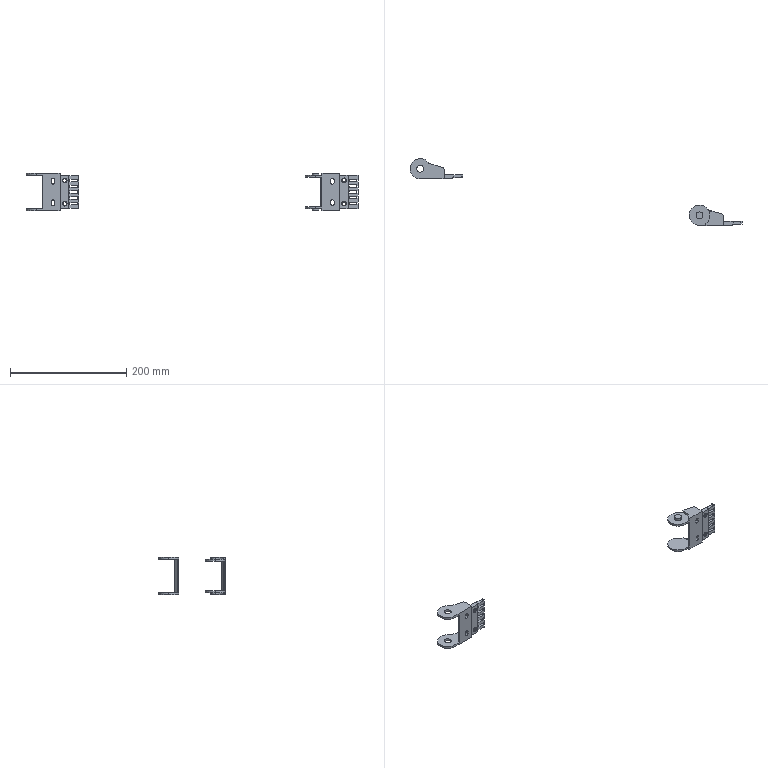Part | SolidWorks | features AEMSimFeature 1 | 4 solids | 238 faces | box 570.077 x 115 x 65.1 mm | volume 63458 mm3 | plane 160 | cylinder 70 | cone 8 | commonest cylinder face diameters 8 x24 6 x12 6.2 x8 35 x8 11.95 x4 12.1 x4